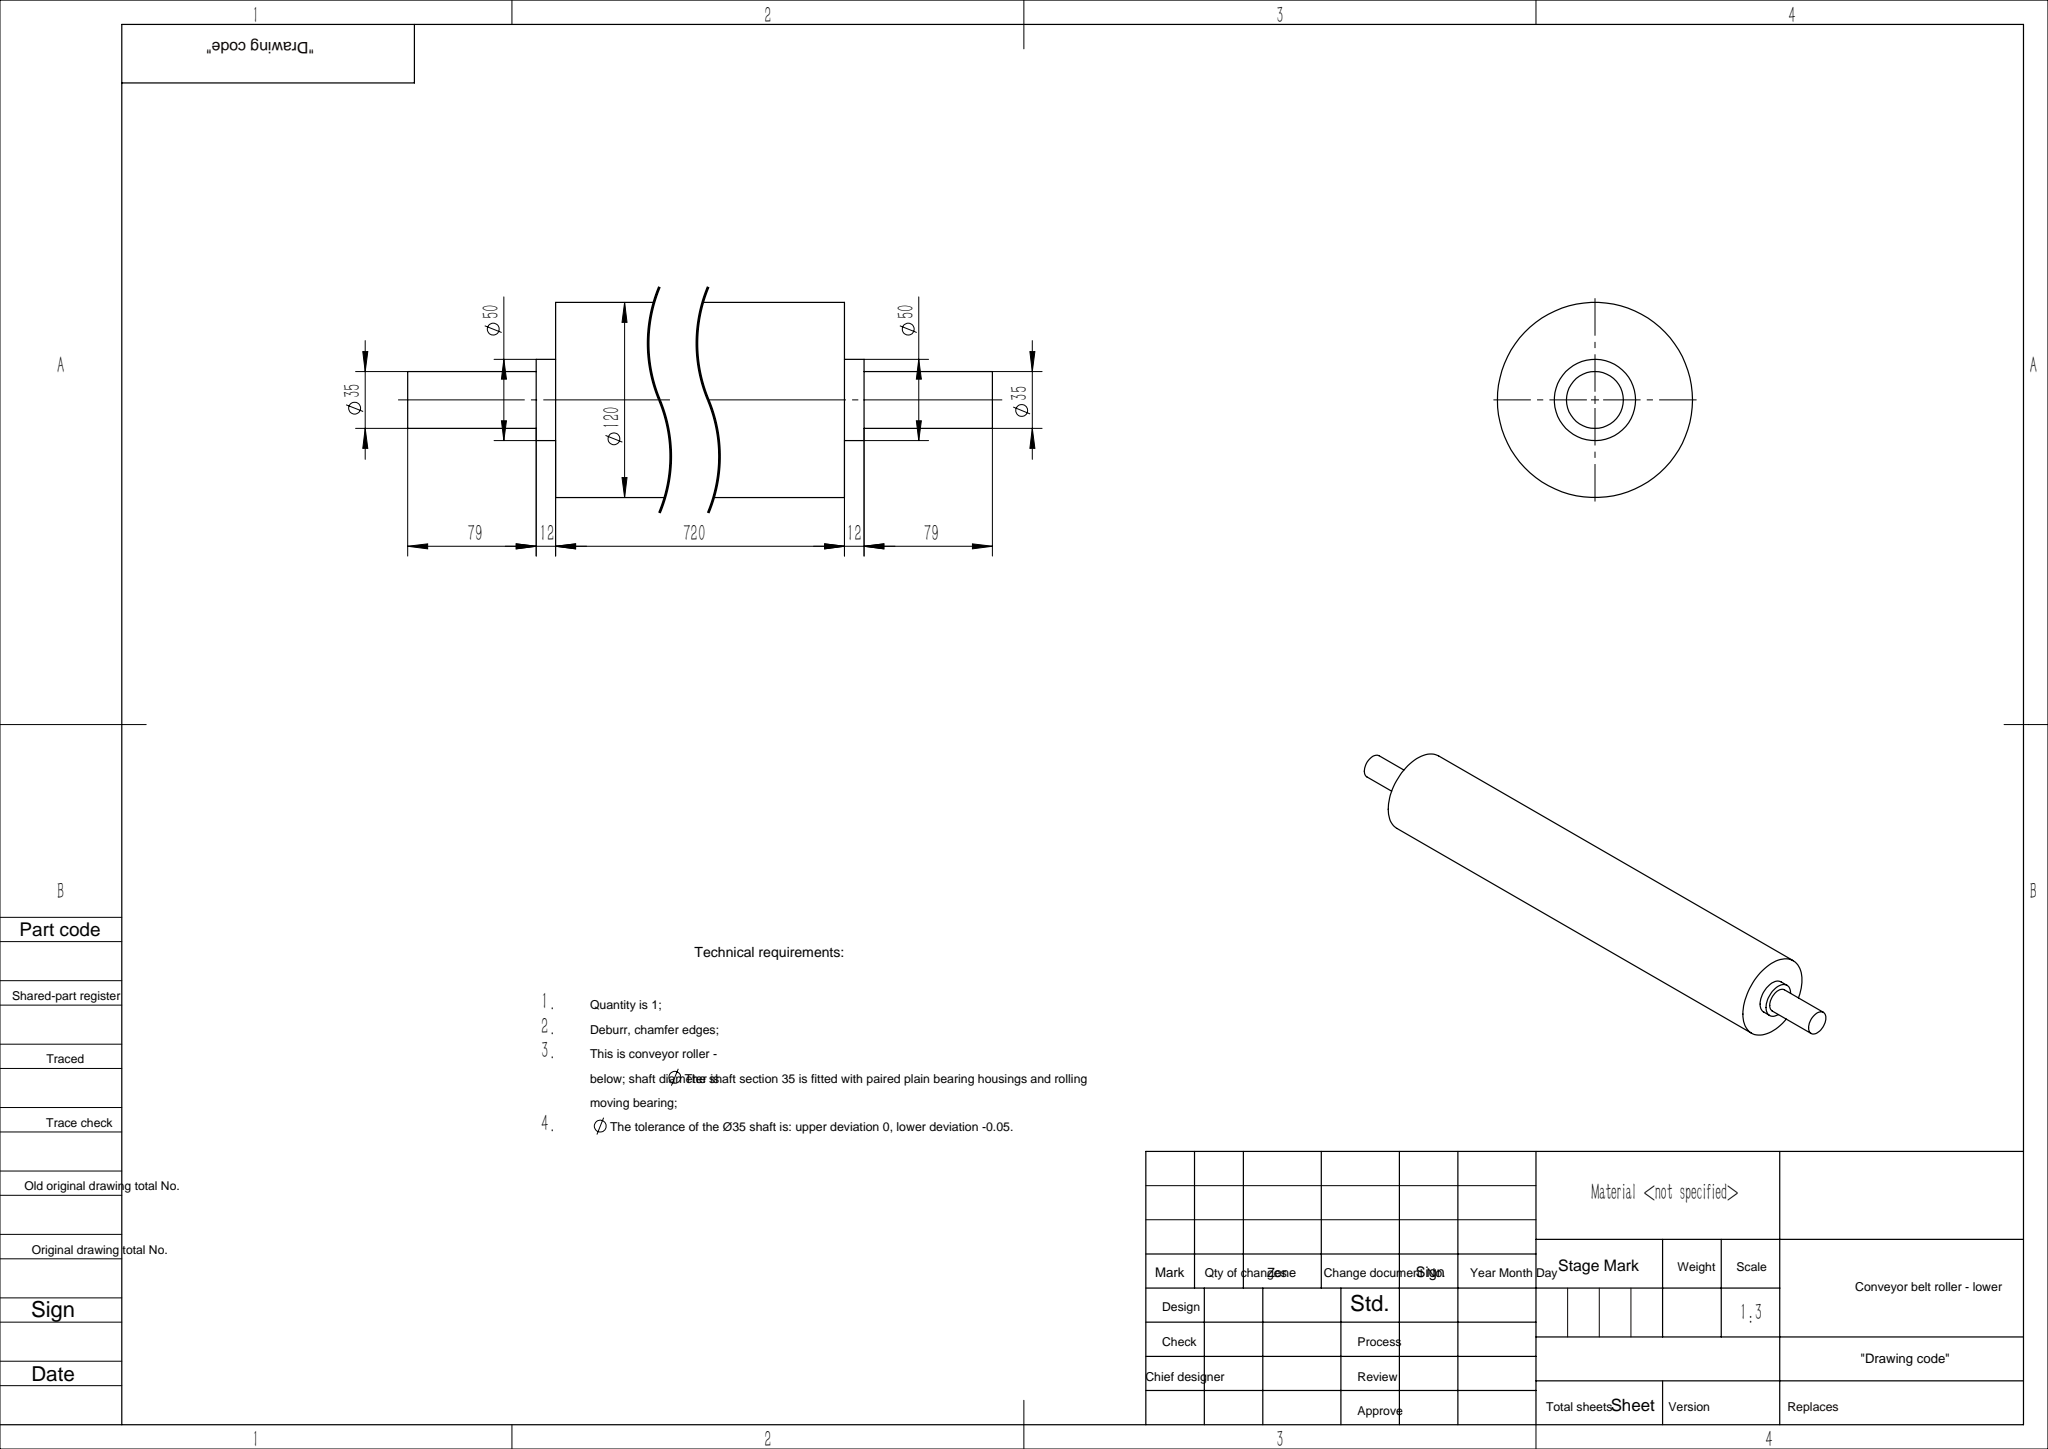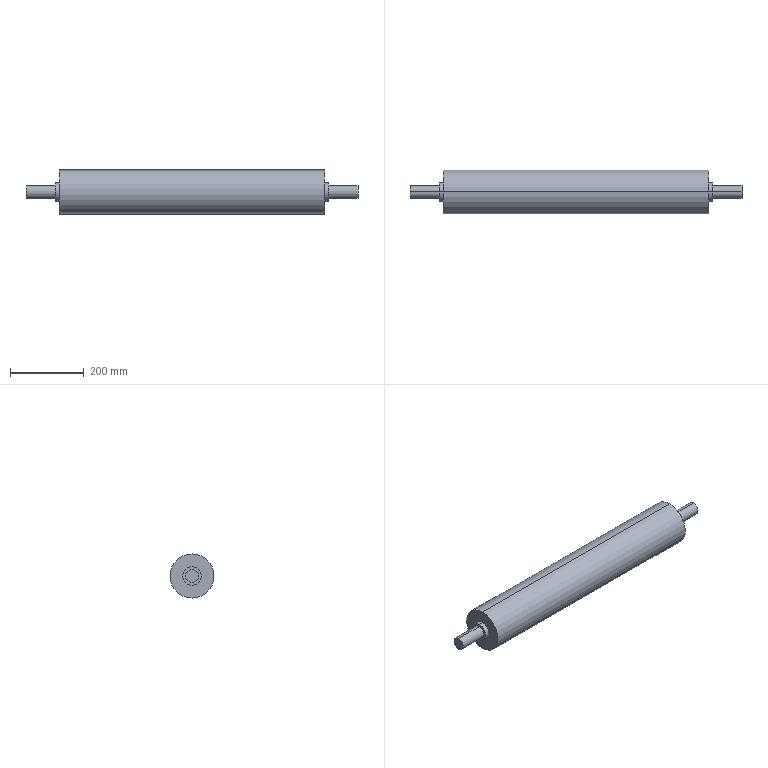Part | SolidWorks | features Revolution 1 | 1 solid | 16 faces | box 902 x 120 x 120 mm | volume 8342146 mm3 | cylinder 10 | plane 6 | commonest cylinder face diameters 35 x4 50 x4 120 x2
STEP:
#1=CARTESIAN_POINT('',(372.,0.,25.));
#2=VERTEX_POINT('',#1);
#3=CARTESIAN_POINT('',(372.,0.,-25.));
#4=VERTEX_POINT('',#3);
#5=CARTESIAN_POINT('',(372.,0.,0.));
#6=DIRECTION('',(-1.,0.,0.));
#7=DIRECTION('',(0.,0.,1.));
#8=AXIS2_PLACEMENT_3D('',#5,#6,#7);
#9=CIRCLE('',#8,25.);
#10=EDGE_CURVE('',#2,#4,#9,.T.);
#11=ORIENTED_EDGE('',*,*,#10,.T.);
#12=CARTESIAN_POINT('',(360.,0.,-25.));
#13=VERTEX_POINT('',#12);
#14=CARTESIAN_POINT('',(-451.,0.,-25.));
#15=DIRECTION('',(-1.,0.,0.));
#16=VECTOR('',#15,1000.);
#17=LINE('',#14,#16);
#18=EDGE_CURVE('',#4,#13,#17,.T.);
#19=ORIENTED_EDGE('',*,*,#18,.T.);
#20=CARTESIAN_POINT('',(360.,0.,25.));
#21=VERTEX_POINT('',#20);
#22=CARTESIAN_POINT('',(360.,0.,0.));
#23=DIRECTION('',(-1.,0.,0.));
#24=DIRECTION('',(0.,0.,1.));
#25=AXIS2_PLACEMENT_3D('',#22,#23,#24);
#26=CIRCLE('',#25,25.);
#27=EDGE_CURVE('',#21,#13,#26,.T.);
#28=ORIENTED_EDGE('',*,*,#27,.F.);
#29=CARTESIAN_POINT('',(-451.,0.,25.));
#30=DIRECTION('',(-1.,0.,0.));
#31=VECTOR('',#30,1000.);
#32=LINE('',#29,#31);
#33=EDGE_CURVE('',#2,#21,#32,.T.);
#34=ORIENTED_EDGE('',*,*,#33,.F.);
#35=EDGE_LOOP('',(#11,#19,#28,#34));
#36=FACE_OUTER_BOUND('',#35,.T.);
#37=CARTESIAN_POINT('',(-451.,0.,0.));
#38=DIRECTION('',(-1.,0.,0.));
#39=DIRECTION('',(0.,0.,1.));
#40=AXIS2_PLACEMENT_3D('',#37,#38,#39);
#41=CYLINDRICAL_SURFACE('',#40,25.);
#42=ADVANCED_FACE('',(#36),#41,.T.);
#43=CARTESIAN_POINT('',(451.,0.,17.5));
#44=VERTEX_POINT('',#43);
#45=CARTESIAN_POINT('',(451.,0.,-17.5));
#46=VERTEX_POINT('',#45);
#47=CARTESIAN_POINT('',(451.,0.,0.));
#48=DIRECTION('',(-1.,0.,0.));
#49=DIRECTION('',(0.,0.,1.));
#50=AXIS2_PLACEMENT_3D('',#47,#48,#49);
#51=CIRCLE('',#50,17.5);
#52=EDGE_CURVE('',#44,#46,#51,.T.);
#53=ORIENTED_EDGE('',*,*,#52,.T.);
#54=CARTESIAN_POINT('',(372.,0.,-17.5));
#55=VERTEX_POINT('',#54);
#56=CARTESIAN_POINT('',(-451.,0.,-17.5));
#57=DIRECTION('',(-1.,0.,0.));
#58=VECTOR('',#57,1000.);
#59=LINE('',#56,#58);
#60=EDGE_CURVE('',#46,#55,#59,.T.);
#61=ORIENTED_EDGE('',*,*,#60,.T.);
#62=CARTESIAN_POINT('',(372.,0.,17.5));
#63=VERTEX_POINT('',#62);
#64=CARTESIAN_POINT('',(372.,0.,0.));
#65=DIRECTION('',(-1.,0.,0.));
#66=DIRECTION('',(0.,0.,1.));
#67=AXIS2_PLACEMENT_3D('',#64,#65,#66);
#68=CIRCLE('',#67,17.5);
#69=EDGE_CURVE('',#63,#55,#68,.T.);
#70=ORIENTED_EDGE('',*,*,#69,.F.);
#71=CARTESIAN_POINT('',(-451.,0.,17.5));
#72=DIRECTION('',(-1.,0.,0.));
#73=VECTOR('',#72,1000.);
#74=LINE('',#71,#73);
#75=EDGE_CURVE('',#44,#63,#74,.T.);
#76=ORIENTED_EDGE('',*,*,#75,.F.);
#77=EDGE_LOOP('',(#53,#61,#70,#76));
#78=FACE_OUTER_BOUND('',#77,.T.);
#79=CARTESIAN_POINT('',(-451.,0.,0.));
#80=DIRECTION('',(-1.,0.,0.));
#81=DIRECTION('',(0.,0.,1.));
#82=AXIS2_PLACEMENT_3D('',#79,#80,#81);
#83=CYLINDRICAL_SURFACE('',#82,17.5);
#84=ADVANCED_FACE('',(#78),#83,.T.);
#85=CARTESIAN_POINT('',(-372.,0.,17.5));
#86=VERTEX_POINT('',#85);
#87=CARTESIAN_POINT('',(-372.,0.,-17.5));
#88=VERTEX_POINT('',#87);
#89=CARTESIAN_POINT('',(-372.,0.,0.));
#90=DIRECTION('',(-1.,0.,0.));
#91=DIRECTION('',(0.,0.,1.));
#92=AXIS2_PLACEMENT_3D('',#89,#90,#91);
#93=CIRCLE('',#92,17.5);
#94=EDGE_CURVE('',#86,#88,#93,.T.);
#95=ORIENTED_EDGE('',*,*,#94,.T.);
#96=CARTESIAN_POINT('',(-451.,0.,-17.5));
#97=VERTEX_POINT('',#96);
#98=CARTESIAN_POINT('',(-451.,0.,-17.5));
#99=DIRECTION('',(-1.,0.,0.));
#100=VECTOR('',#99,1000.);
#101=LINE('',#98,#100);
#102=EDGE_CURVE('',#88,#97,#101,.T.);
#103=ORIENTED_EDGE('',*,*,#102,.T.);
#104=CARTESIAN_POINT('',(-451.,0.,17.5));
#105=VERTEX_POINT('',#104);
#106=CARTESIAN_POINT('',(-451.,0.,0.));
#107=DIRECTION('',(-1.,0.,0.));
#108=DIRECTION('',(0.,0.,1.));
#109=AXIS2_PLACEMENT_3D('',#106,#107,#108);
#110=CIRCLE('',#109,17.5);
#111=EDGE_CURVE('',#105,#97,#110,.T.);
#112=ORIENTED_EDGE('',*,*,#111,.F.);
#113=CARTESIAN_POINT('',(-451.,0.,17.5));
#114=DIRECTION('',(-1.,0.,0.));
#115=VECTOR('',#114,1000.);
#116=LINE('',#113,#115);
#117=EDGE_CURVE('',#86,#105,#116,.T.);
#118=ORIENTED_EDGE('',*,*,#117,.F.);
#119=EDGE_LOOP('',(#95,#103,#112,#118));
#120=FACE_OUTER_BOUND('',#119,.T.);
#121=CARTESIAN_POINT('',(-451.,0.,0.));
#122=DIRECTION('',(-1.,0.,0.));
#123=DIRECTION('',(0.,0.,1.));
#124=AXIS2_PLACEMENT_3D('',#121,#122,#123);
#125=CYLINDRICAL_SURFACE('',#124,17.5);
#126=ADVANCED_FACE('',(#120),#125,.T.);
#127=CARTESIAN_POINT('',(-360.,0.,25.));
#128=VERTEX_POINT('',#127);
#129=CARTESIAN_POINT('',(-360.,0.,-25.));
#130=VERTEX_POINT('',#129);
#131=CARTESIAN_POINT('',(-360.,0.,0.));
#132=DIRECTION('',(-1.,0.,0.));
#133=DIRECTION('',(0.,0.,1.));
#134=AXIS2_PLACEMENT_3D('',#131,#132,#133);
#135=CIRCLE('',#134,25.);
#136=EDGE_CURVE('',#128,#130,#135,.T.);
#137=ORIENTED_EDGE('',*,*,#136,.T.);
#138=CARTESIAN_POINT('',(-372.,0.,-25.));
#139=VERTEX_POINT('',#138);
#140=CARTESIAN_POINT('',(-451.,0.,-25.));
#141=DIRECTION('',(-1.,0.,0.));
#142=VECTOR('',#141,1000.);
#143=LINE('',#140,#142);
#144=EDGE_CURVE('',#130,#139,#143,.T.);
#145=ORIENTED_EDGE('',*,*,#144,.T.);
#146=CARTESIAN_POINT('',(-372.,0.,25.));
#147=VERTEX_POINT('',#146);
#148=CARTESIAN_POINT('',(-372.,0.,0.));
#149=DIRECTION('',(-1.,0.,0.));
#150=DIRECTION('',(0.,0.,1.));
#151=AXIS2_PLACEMENT_3D('',#148,#149,#150);
#152=CIRCLE('',#151,25.);
#153=EDGE_CURVE('',#147,#139,#152,.T.);
#154=ORIENTED_EDGE('',*,*,#153,.F.);
#155=CARTESIAN_POINT('',(-451.,0.,25.));
#156=DIRECTION('',(-1.,0.,0.));
#157=VECTOR('',#156,1000.);
#158=LINE('',#155,#157);
#159=EDGE_CURVE('',#128,#147,#158,.T.);
#160=ORIENTED_EDGE('',*,*,#159,.F.);
#161=EDGE_LOOP('',(#137,#145,#154,#160));
#162=FACE_OUTER_BOUND('',#161,.T.);
#163=CARTESIAN_POINT('',(-451.,0.,0.));
#164=DIRECTION('',(-1.,0.,0.));
#165=DIRECTION('',(0.,0.,1.));
#166=AXIS2_PLACEMENT_3D('',#163,#164,#165);
#167=CYLINDRICAL_SURFACE('',#166,25.);
#168=ADVANCED_FACE('',(#162),#167,.T.);
#169=CARTESIAN_POINT('',(360.,0.,60.));
#170=VERTEX_POINT('',#169);
#171=CARTESIAN_POINT('',(360.,0.,-60.));
#172=VERTEX_POINT('',#171);
#173=CARTESIAN_POINT('',(360.,0.,0.));
#174=DIRECTION('',(-1.,0.,0.));
#175=DIRECTION('',(0.,0.,1.));
#176=AXIS2_PLACEMENT_3D('',#173,#174,#175);
#177=CIRCLE('',#176,60.);
#178=EDGE_CURVE('',#170,#172,#177,.T.);
#179=ORIENTED_EDGE('',*,*,#178,.T.);
#180=CARTESIAN_POINT('',(-360.,0.,-60.));
#181=VERTEX_POINT('',#180);
#182=CARTESIAN_POINT('',(-451.,0.,-60.));
#183=DIRECTION('',(-1.,0.,0.));
#184=VECTOR('',#183,1000.);
#185=LINE('',#182,#184);
#186=EDGE_CURVE('',#172,#181,#185,.T.);
#187=ORIENTED_EDGE('',*,*,#186,.T.);
#188=CARTESIAN_POINT('',(-360.,0.,60.));
#189=VERTEX_POINT('',#188);
#190=CARTESIAN_POINT('',(-360.,0.,0.));
#191=DIRECTION('',(-1.,0.,0.));
#192=DIRECTION('',(0.,0.,1.));
#193=AXIS2_PLACEMENT_3D('',#190,#191,#192);
#194=CIRCLE('',#193,60.);
#195=EDGE_CURVE('',#189,#181,#194,.T.);
#196=ORIENTED_EDGE('',*,*,#195,.F.);
#197=CARTESIAN_POINT('',(-451.,0.,60.));
#198=DIRECTION('',(-1.,0.,0.));
#199=VECTOR('',#198,1000.);
#200=LINE('',#197,#199);
#201=EDGE_CURVE('',#170,#189,#200,.T.);
#202=ORIENTED_EDGE('',*,*,#201,.F.);
#203=EDGE_LOOP('',(#179,#187,#196,#202));
#204=FACE_OUTER_BOUND('',#203,.T.);
#205=CARTESIAN_POINT('',(-451.,0.,0.));
#206=DIRECTION('',(-1.,0.,0.));
#207=DIRECTION('',(0.,0.,1.));
#208=AXIS2_PLACEMENT_3D('',#205,#206,#207);
#209=CYLINDRICAL_SURFACE('',#208,60.);
#210=ADVANCED_FACE('',(#204),#209,.T.);
#211=ORIENTED_EDGE('',*,*,#178,.F.);
#212=CARTESIAN_POINT('',(360.,0.,0.));
#213=DIRECTION('',(-1.,0.,0.));
#214=DIRECTION('',(0.,0.,1.));
#215=AXIS2_PLACEMENT_3D('',#212,#213,#214);
#216=CIRCLE('',#215,60.);
#217=EDGE_CURVE('',#172,#170,#216,.T.);
#218=ORIENTED_EDGE('',*,*,#217,.F.);
#219=EDGE_LOOP('',(#211,#218));
#220=FACE_OUTER_BOUND('',#219,.T.);
#221=ORIENTED_EDGE('',*,*,#27,.T.);
#222=CARTESIAN_POINT('',(360.,0.,0.));
#223=DIRECTION('',(-1.,0.,0.));
#224=DIRECTION('',(0.,0.,1.));
#225=AXIS2_PLACEMENT_3D('',#222,#223,#224);
#226=CIRCLE('',#225,25.);
#227=EDGE_CURVE('',#13,#21,#226,.T.);
#228=ORIENTED_EDGE('',*,*,#227,.T.);
#229=EDGE_LOOP('',(#221,#228));
#230=FACE_BOUND('',#229,.T.);
#231=CARTESIAN_POINT('',(360.,60.,0.));
#232=DIRECTION('',(-1.,0.,0.));
#233=DIRECTION('',(0.,0.,1.));
#234=AXIS2_PLACEMENT_3D('',#231,#232,#233);
#235=PLANE('',#234);
#236=ADVANCED_FACE('',(#220,#230),#235,.F.);
#237=ORIENTED_EDGE('',*,*,#186,.F.);
#238=ORIENTED_EDGE('',*,*,#217,.T.);
#239=ORIENTED_EDGE('',*,*,#201,.T.);
#240=CARTESIAN_POINT('',(-360.,0.,0.));
#241=DIRECTION('',(-1.,0.,0.));
#242=DIRECTION('',(0.,0.,1.));
#243=AXIS2_PLACEMENT_3D('',#240,#241,#242);
#244=CIRCLE('',#243,60.);
#245=EDGE_CURVE('',#181,#189,#244,.T.);
#246=ORIENTED_EDGE('',*,*,#245,.F.);
#247=EDGE_LOOP('',(#237,#238,#239,#246));
#248=FACE_OUTER_BOUND('',#247,.T.);
#249=CARTESIAN_POINT('',(-451.,0.,0.));
#250=DIRECTION('',(-1.,0.,0.));
#251=DIRECTION('',(0.,0.,1.));
#252=AXIS2_PLACEMENT_3D('',#249,#250,#251);
#253=CYLINDRICAL_SURFACE('',#252,60.);
#254=ADVANCED_FACE('',(#248),#253,.T.);
#255=ORIENTED_EDGE('',*,*,#136,.F.);
#256=CARTESIAN_POINT('',(-360.,0.,0.));
#257=DIRECTION('',(-1.,0.,0.));
#258=DIRECTION('',(0.,0.,1.));
#259=AXIS2_PLACEMENT_3D('',#256,#257,#258);
#260=CIRCLE('',#259,25.);
#261=EDGE_CURVE('',#130,#128,#260,.T.);
#262=ORIENTED_EDGE('',*,*,#261,.F.);
#263=EDGE_LOOP('',(#255,#262));
#264=FACE_BOUND('',#263,.T.);
#265=ORIENTED_EDGE('',*,*,#195,.T.);
#266=ORIENTED_EDGE('',*,*,#245,.T.);
#267=EDGE_LOOP('',(#265,#266));
#268=FACE_OUTER_BOUND('',#267,.T.);
#269=CARTESIAN_POINT('',(-360.,60.,0.));
#270=DIRECTION('',(1.,0.,0.));
#271=DIRECTION('',(0.,0.,-1.));
#272=AXIS2_PLACEMENT_3D('',#269,#270,#271);
#273=PLANE('',#272);
#274=ADVANCED_FACE('',(#264,#268),#273,.F.);
#275=ORIENTED_EDGE('',*,*,#144,.F.);
#276=ORIENTED_EDGE('',*,*,#261,.T.);
#277=ORIENTED_EDGE('',*,*,#159,.T.);
#278=CARTESIAN_POINT('',(-372.,0.,0.));
#279=DIRECTION('',(-1.,0.,0.));
#280=DIRECTION('',(0.,0.,1.));
#281=AXIS2_PLACEMENT_3D('',#278,#279,#280);
#282=CIRCLE('',#281,25.);
#283=EDGE_CURVE('',#139,#147,#282,.T.);
#284=ORIENTED_EDGE('',*,*,#283,.F.);
#285=EDGE_LOOP('',(#275,#276,#277,#284));
#286=FACE_OUTER_BOUND('',#285,.T.);
#287=CARTESIAN_POINT('',(-451.,0.,0.));
#288=DIRECTION('',(-1.,0.,0.));
#289=DIRECTION('',(0.,0.,1.));
#290=AXIS2_PLACEMENT_3D('',#287,#288,#289);
#291=CYLINDRICAL_SURFACE('',#290,25.);
#292=ADVANCED_FACE('',(#286),#291,.T.);
#293=ORIENTED_EDGE('',*,*,#94,.F.);
#294=CARTESIAN_POINT('',(-372.,0.,0.));
#295=DIRECTION('',(-1.,0.,0.));
#296=DIRECTION('',(0.,0.,1.));
#297=AXIS2_PLACEMENT_3D('',#294,#295,#296);
#298=CIRCLE('',#297,17.5);
#299=EDGE_CURVE('',#88,#86,#298,.T.);
#300=ORIENTED_EDGE('',*,*,#299,.F.);
#301=EDGE_LOOP('',(#293,#300));
#302=FACE_BOUND('',#301,.T.);
#303=ORIENTED_EDGE('',*,*,#153,.T.);
#304=ORIENTED_EDGE('',*,*,#283,.T.);
#305=EDGE_LOOP('',(#303,#304));
#306=FACE_OUTER_BOUND('',#305,.T.);
#307=CARTESIAN_POINT('',(-372.,25.,0.));
#308=DIRECTION('',(1.,0.,0.));
#309=DIRECTION('',(0.,0.,-1.));
#310=AXIS2_PLACEMENT_3D('',#307,#308,#309);
#311=PLANE('',#310);
#312=ADVANCED_FACE('',(#302,#306),#311,.F.);
#313=ORIENTED_EDGE('',*,*,#102,.F.);
#314=ORIENTED_EDGE('',*,*,#299,.T.);
#315=ORIENTED_EDGE('',*,*,#117,.T.);
#316=CARTESIAN_POINT('',(-451.,0.,0.));
#317=DIRECTION('',(-1.,0.,0.));
#318=DIRECTION('',(0.,0.,1.));
#319=AXIS2_PLACEMENT_3D('',#316,#317,#318);
#320=CIRCLE('',#319,17.5);
#321=EDGE_CURVE('',#97,#105,#320,.T.);
#322=ORIENTED_EDGE('',*,*,#321,.F.);
#323=EDGE_LOOP('',(#313,#314,#315,#322));
#324=FACE_OUTER_BOUND('',#323,.T.);
#325=CARTESIAN_POINT('',(-451.,0.,0.));
#326=DIRECTION('',(-1.,0.,0.));
#327=DIRECTION('',(0.,0.,1.));
#328=AXIS2_PLACEMENT_3D('',#325,#326,#327);
#329=CYLINDRICAL_SURFACE('',#328,17.5);
#330=ADVANCED_FACE('',(#324),#329,.T.);
#331=ORIENTED_EDGE('',*,*,#111,.T.);
#332=ORIENTED_EDGE('',*,*,#321,.T.);
#333=EDGE_LOOP('',(#331,#332));
#334=FACE_OUTER_BOUND('',#333,.T.);
#335=CARTESIAN_POINT('',(-451.,17.5,0.));
#336=DIRECTION('',(1.,0.,0.));
#337=DIRECTION('',(0.,0.,-1.));
#338=AXIS2_PLACEMENT_3D('',#335,#336,#337);
#339=PLANE('',#338);
#340=ADVANCED_FACE('',(#334),#339,.F.);
#341=ORIENTED_EDGE('',*,*,#52,.F.);
#342=CARTESIAN_POINT('',(451.,0.,0.));
#343=DIRECTION('',(-1.,0.,0.));
#344=DIRECTION('',(0.,0.,1.));
#345=AXIS2_PLACEMENT_3D('',#342,#343,#344);
#346=CIRCLE('',#345,17.5);
#347=EDGE_CURVE('',#46,#44,#346,.T.);
#348=ORIENTED_EDGE('',*,*,#347,.F.);
#349=EDGE_LOOP('',(#341,#348));
#350=FACE_OUTER_BOUND('',#349,.T.);
#351=CARTESIAN_POINT('',(451.,17.5,0.));
#352=DIRECTION('',(-1.,0.,0.));
#353=DIRECTION('',(0.,0.,1.));
#354=AXIS2_PLACEMENT_3D('',#351,#352,#353);
#355=PLANE('',#354);
#356=ADVANCED_FACE('',(#350),#355,.F.);
#357=ORIENTED_EDGE('',*,*,#60,.F.);
#358=ORIENTED_EDGE('',*,*,#347,.T.);
#359=ORIENTED_EDGE('',*,*,#75,.T.);
#360=CARTESIAN_POINT('',(372.,0.,0.));
#361=DIRECTION('',(-1.,0.,0.));
#362=DIRECTION('',(0.,0.,1.));
#363=AXIS2_PLACEMENT_3D('',#360,#361,#362);
#364=CIRCLE('',#363,17.5);
#365=EDGE_CURVE('',#55,#63,#364,.T.);
#366=ORIENTED_EDGE('',*,*,#365,.F.);
#367=EDGE_LOOP('',(#357,#358,#359,#366));
#368=FACE_OUTER_BOUND('',#367,.T.);
#369=CARTESIAN_POINT('',(-451.,0.,0.));
#370=DIRECTION('',(-1.,0.,0.));
#371=DIRECTION('',(0.,0.,1.));
#372=AXIS2_PLACEMENT_3D('',#369,#370,#371);
#373=CYLINDRICAL_SURFACE('',#372,17.5);
#374=ADVANCED_FACE('',(#368),#373,.T.);
#375=ORIENTED_EDGE('',*,*,#10,.F.);
#376=CARTESIAN_POINT('',(372.,0.,0.));
#377=DIRECTION('',(-1.,0.,0.));
#378=DIRECTION('',(0.,0.,1.));
#379=AXIS2_PLACEMENT_3D('',#376,#377,#378);
#380=CIRCLE('',#379,25.);
#381=EDGE_CURVE('',#4,#2,#380,.T.);
#382=ORIENTED_EDGE('',*,*,#381,.F.);
#383=EDGE_LOOP('',(#375,#382));
#384=FACE_OUTER_BOUND('',#383,.T.);
#385=ORIENTED_EDGE('',*,*,#69,.T.);
#386=ORIENTED_EDGE('',*,*,#365,.T.);
#387=EDGE_LOOP('',(#385,#386));
#388=FACE_BOUND('',#387,.T.);
#389=CARTESIAN_POINT('',(372.,25.,0.));
#390=DIRECTION('',(-1.,0.,0.));
#391=DIRECTION('',(0.,0.,1.));
#392=AXIS2_PLACEMENT_3D('',#389,#390,#391);
#393=PLANE('',#392);
#394=ADVANCED_FACE('',(#384,#388),#393,.F.);
#395=ORIENTED_EDGE('',*,*,#18,.F.);
#396=ORIENTED_EDGE('',*,*,#381,.T.);
#397=ORIENTED_EDGE('',*,*,#33,.T.);
#398=ORIENTED_EDGE('',*,*,#227,.F.);
#399=EDGE_LOOP('',(#395,#396,#397,#398));
#400=FACE_OUTER_BOUND('',#399,.T.);
#401=CARTESIAN_POINT('',(-451.,0.,0.));
#402=DIRECTION('',(-1.,0.,0.));
#403=DIRECTION('',(0.,0.,1.));
#404=AXIS2_PLACEMENT_3D('',#401,#402,#403);
#405=CYLINDRICAL_SURFACE('',#404,25.);
#406=ADVANCED_FACE('',(#400),#405,.T.);
#407=CLOSED_SHELL('',(#42,#84,#126,#168,#210,#236,#254,#274,#292,#312,#330,#340,#356,#374,#394,#406));
#408=MANIFOLD_SOLID_BREP('',#407);
#409=CARTESIAN_POINT('',(0.,0.,0.));
#410=DIRECTION('',(0.,0.,1.));
#411=DIRECTION('',(1.,0.,0.));
#412=AXIS2_PLACEMENT_3D('',#409,#410,#411);
#413=(LENGTH_UNIT()NAMED_UNIT(*)SI_UNIT(.MILLI.,.METRE.));
#414=UNCERTAINTY_MEASURE_WITH_UNIT(LENGTH_MEASURE(0.00001),#413,'','');
#415=(NAMED_UNIT(*)PLANE_ANGLE_UNIT()SI_UNIT($,.RADIAN.));
#416=(NAMED_UNIT(*)SI_UNIT($,.STERADIAN.)SOLID_ANGLE_UNIT());
#417=(GEOMETRIC_REPRESENTATION_CONTEXT(3)GLOBAL_UNCERTAINTY_ASSIGNED_CONTEXT((#414))GLOBAL_UNIT_ASSIGNED_CONTEXT((#413,#415,#416))REPRESENTATION_CONTEXT('',''));
#418=ADVANCED_BREP_SHAPE_REPRESENTATION('',(#408,#412),#417);